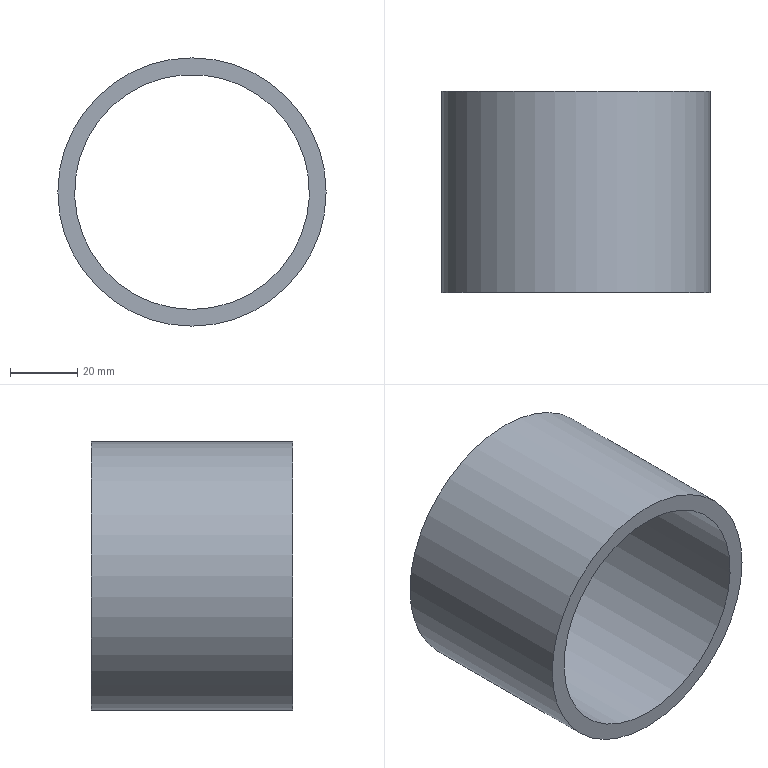Part | NX | features DATUM_CSYS 2, EXTRUDE 1, SKETCH 1 | 1 solid | 4 faces | box 80 x 60 x 80 mm | volume 70686 mm3 | plane 2 | cylinder 2 | commonest cylinder face diameters 70 x1 80 x1
STEP:
#1=CARTESIAN_POINT('',(0.,30.,-35.));
#2=VERTEX_POINT('',#1);
#3=CARTESIAN_POINT('',(0.,30.,0.));
#4=DIRECTION('',(0.,-1.,0.));
#5=DIRECTION('',(0.,0.,-1.));
#6=AXIS2_PLACEMENT_3D('',#3,#4,#5);
#7=CIRCLE('',#6,35.);
#8=EDGE_CURVE('',#2,#2,#7,.T.);
#9=ORIENTED_EDGE('',*,*,#8,.T.);
#10=EDGE_LOOP('',(#9));
#11=FACE_BOUND('',#10,.T.);
#12=CARTESIAN_POINT('',(40.,30.,0.));
#13=VERTEX_POINT('',#12);
#14=CARTESIAN_POINT('',(0.,30.,0.));
#15=DIRECTION('',(0.,-1.,0.));
#16=DIRECTION('',(1.,0.,0.));
#17=AXIS2_PLACEMENT_3D('',#14,#15,#16);
#18=CIRCLE('',#17,40.);
#19=EDGE_CURVE('',#13,#13,#18,.T.);
#20=ORIENTED_EDGE('',*,*,#19,.F.);
#21=EDGE_LOOP('',(#20));
#22=FACE_BOUND('',#21,.T.);
#23=CARTESIAN_POINT('',(0.,30.,0.));
#24=DIRECTION('',(0.,1.,0.));
#25=DIRECTION('',(0.,0.,1.));
#26=AXIS2_PLACEMENT_3D('',#23,#24,#25);
#27=PLANE('',#26);
#28=ADVANCED_FACE('',(#11,#22),#27,.T.);
#29=CARTESIAN_POINT('',(0.,-30.,-35.));
#30=VERTEX_POINT('',#29);
#31=CARTESIAN_POINT('',(0.,-30.,0.));
#32=DIRECTION('',(0.,-1.,0.));
#33=DIRECTION('',(0.,0.,-1.));
#34=AXIS2_PLACEMENT_3D('',#31,#32,#33);
#35=CIRCLE('',#34,35.);
#36=EDGE_CURVE('',#30,#30,#35,.T.);
#37=ORIENTED_EDGE('',*,*,#36,.F.);
#38=EDGE_LOOP('',(#37));
#39=FACE_BOUND('',#38,.T.);
#40=CARTESIAN_POINT('',(40.,-30.,0.));
#41=VERTEX_POINT('',#40);
#42=CARTESIAN_POINT('',(0.,-30.,0.));
#43=DIRECTION('',(0.,-1.,0.));
#44=DIRECTION('',(1.,0.,0.));
#45=AXIS2_PLACEMENT_3D('',#42,#43,#44);
#46=CIRCLE('',#45,40.);
#47=EDGE_CURVE('',#41,#41,#46,.T.);
#48=ORIENTED_EDGE('',*,*,#47,.T.);
#49=EDGE_LOOP('',(#48));
#50=FACE_BOUND('',#49,.T.);
#51=CARTESIAN_POINT('',(0.,-30.,0.));
#52=DIRECTION('',(0.,1.,0.));
#53=DIRECTION('',(0.,0.,1.));
#54=AXIS2_PLACEMENT_3D('',#51,#52,#53);
#55=PLANE('',#54);
#56=ADVANCED_FACE('',(#39,#50),#55,.F.);
#57=ORIENTED_EDGE('',*,*,#8,.F.);
#58=EDGE_LOOP('',(#57));
#59=FACE_BOUND('',#58,.T.);
#60=ORIENTED_EDGE('',*,*,#36,.T.);
#61=EDGE_LOOP('',(#60));
#62=FACE_BOUND('',#61,.T.);
#63=CARTESIAN_POINT('',(0.,30.,0.));
#64=DIRECTION('',(0.,-1.,0.));
#65=DIRECTION('',(0.,0.,-1.));
#66=AXIS2_PLACEMENT_3D('',#63,#64,#65);
#67=CYLINDRICAL_SURFACE('',#66,35.);
#68=ADVANCED_FACE('',(#59,#62),#67,.F.);
#69=ORIENTED_EDGE('',*,*,#19,.T.);
#70=EDGE_LOOP('',(#69));
#71=FACE_BOUND('',#70,.T.);
#72=ORIENTED_EDGE('',*,*,#47,.F.);
#73=EDGE_LOOP('',(#72));
#74=FACE_BOUND('',#73,.T.);
#75=CARTESIAN_POINT('',(0.,30.,0.));
#76=DIRECTION('',(0.,-1.,0.));
#77=DIRECTION('',(0.,0.,-1.));
#78=AXIS2_PLACEMENT_3D('',#75,#76,#77);
#79=CYLINDRICAL_SURFACE('',#78,40.);
#80=ADVANCED_FACE('',(#71,#74),#79,.T.);
#81=CLOSED_SHELL('',(#28,#56,#68,#80));
#82=MANIFOLD_SOLID_BREP('',#81);
#83=(LENGTH_UNIT()NAMED_UNIT(*)SI_UNIT(.MILLI.,.METRE.));
#84=UNCERTAINTY_MEASURE_WITH_UNIT(LENGTH_MEASURE(0.00001),#83,'','');
#85=(NAMED_UNIT(*)PLANE_ANGLE_UNIT()SI_UNIT($,.RADIAN.));
#86=(NAMED_UNIT(*)SI_UNIT($,.STERADIAN.)SOLID_ANGLE_UNIT());
#87=(GEOMETRIC_REPRESENTATION_CONTEXT(3)GLOBAL_UNCERTAINTY_ASSIGNED_CONTEXT((#84))GLOBAL_UNIT_ASSIGNED_CONTEXT((#83,#85,#86))REPRESENTATION_CONTEXT('',''));
#88=ADVANCED_BREP_SHAPE_REPRESENTATION('',(#82),#87);